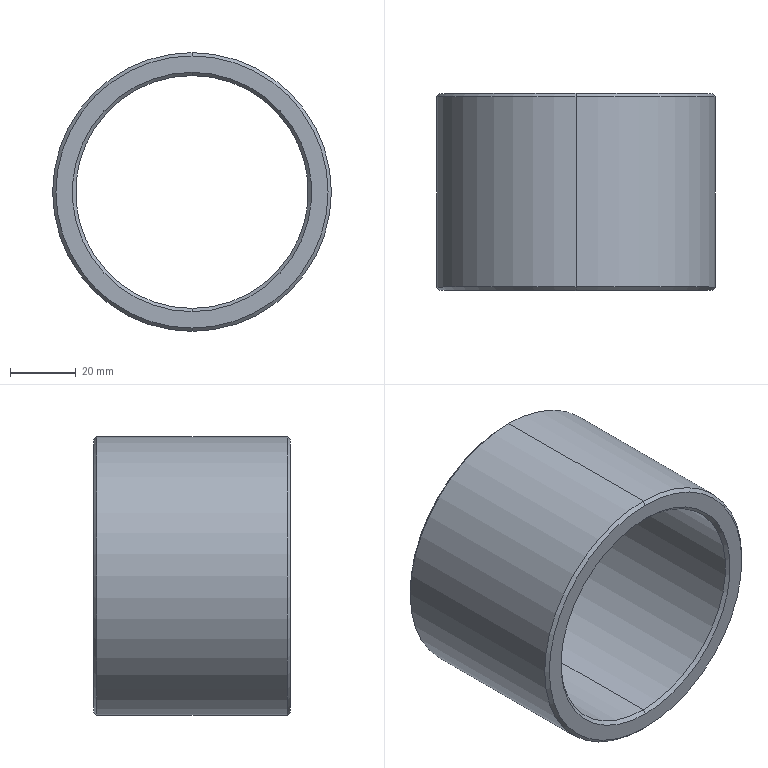Part | SolidWorks | features Chamfer 1, Extrusion 1 | 1 solid | 14 faces | box 85 x 60 x 85 mm | volume 102428 mm3 | cone 8 | cylinder 4 | plane 2 | commonest cylinder face diameters 71 x2 85 x2
STEP:
#1=CARTESIAN_POINT('',(0.,60.,41.5));
#2=VERTEX_POINT('',#1);
#3=CARTESIAN_POINT('',(0.,60.,-41.5));
#4=VERTEX_POINT('',#3);
#5=CARTESIAN_POINT('',(0.,60.,0.));
#6=DIRECTION('',(0.,1.,0.));
#7=DIRECTION('',(0.,0.,1.));
#8=AXIS2_PLACEMENT_3D('',#5,#6,#7);
#9=CIRCLE('',#8,41.5);
#10=EDGE_CURVE('',#2,#4,#9,.T.);
#11=ORIENTED_EDGE('',*,*,#10,.F.);
#12=CARTESIAN_POINT('',(0.,59.,42.5));
#13=VERTEX_POINT('',#12);
#14=CARTESIAN_POINT('',(0.,60.,41.5));
#15=DIRECTION('',(0.,-0.7071,0.7071));
#16=VECTOR('',#15,1000.);
#17=LINE('',#14,#16);
#18=EDGE_CURVE('',#2,#13,#17,.T.);
#19=ORIENTED_EDGE('',*,*,#18,.T.);
#20=CARTESIAN_POINT('',(0.,59.,-42.5));
#21=VERTEX_POINT('',#20);
#22=CARTESIAN_POINT('',(0.,59.,0.));
#23=DIRECTION('',(0.,-1.,0.));
#24=DIRECTION('',(0.,0.,1.));
#25=AXIS2_PLACEMENT_3D('',#22,#23,#24);
#26=CIRCLE('',#25,42.5);
#27=EDGE_CURVE('',#21,#13,#26,.T.);
#28=ORIENTED_EDGE('',*,*,#27,.F.);
#29=CARTESIAN_POINT('',(0.,60.,-41.5));
#30=DIRECTION('',(0.,-0.7071,-0.7071));
#31=VECTOR('',#30,1000.);
#32=LINE('',#29,#31);
#33=EDGE_CURVE('',#4,#21,#32,.T.);
#34=ORIENTED_EDGE('',*,*,#33,.F.);
#35=EDGE_LOOP('',(#11,#19,#28,#34));
#36=FACE_OUTER_BOUND('',#35,.T.);
#37=CARTESIAN_POINT('',(0.,60.,0.));
#38=DIRECTION('',(0.,-1.,0.));
#39=DIRECTION('',(0.,0.,-1.));
#40=AXIS2_PLACEMENT_3D('',#37,#38,#39);
#41=CONICAL_SURFACE('',#40,41.5,0.7854);
#42=ADVANCED_FACE('',(#36),#41,.T.);
#43=CARTESIAN_POINT('',(0.,0.,-41.5));
#44=VERTEX_POINT('',#43);
#45=CARTESIAN_POINT('',(0.,0.,41.5));
#46=VERTEX_POINT('',#45);
#47=CARTESIAN_POINT('',(0.,0.,0.));
#48=DIRECTION('',(0.,-1.,0.));
#49=DIRECTION('',(0.,0.,1.));
#50=AXIS2_PLACEMENT_3D('',#47,#48,#49);
#51=CIRCLE('',#50,41.5);
#52=EDGE_CURVE('',#44,#46,#51,.T.);
#53=ORIENTED_EDGE('',*,*,#52,.F.);
#54=CARTESIAN_POINT('',(0.,1.,-42.5));
#55=VERTEX_POINT('',#54);
#56=CARTESIAN_POINT('',(0.,1.,-42.5));
#57=DIRECTION('',(0.,0.7071,-0.7071));
#58=VECTOR('',#57,1000.);
#59=LINE('',#56,#58);
#60=EDGE_CURVE('',#44,#55,#59,.T.);
#61=ORIENTED_EDGE('',*,*,#60,.T.);
#62=CARTESIAN_POINT('',(0.,1.,42.5));
#63=VERTEX_POINT('',#62);
#64=CARTESIAN_POINT('',(0.,1.,0.));
#65=DIRECTION('',(0.,1.,0.));
#66=DIRECTION('',(0.,0.,1.));
#67=AXIS2_PLACEMENT_3D('',#64,#65,#66);
#68=CIRCLE('',#67,42.5);
#69=EDGE_CURVE('',#63,#55,#68,.T.);
#70=ORIENTED_EDGE('',*,*,#69,.F.);
#71=CARTESIAN_POINT('',(0.,1.,42.5));
#72=DIRECTION('',(0.,0.7071,0.7071));
#73=VECTOR('',#72,1000.);
#74=LINE('',#71,#73);
#75=EDGE_CURVE('',#46,#63,#74,.T.);
#76=ORIENTED_EDGE('',*,*,#75,.F.);
#77=EDGE_LOOP('',(#53,#61,#70,#76));
#78=FACE_OUTER_BOUND('',#77,.T.);
#79=CARTESIAN_POINT('',(0.,1.,0.));
#80=DIRECTION('',(0.,1.,0.));
#81=DIRECTION('',(0.,0.,1.));
#82=AXIS2_PLACEMENT_3D('',#79,#80,#81);
#83=CONICAL_SURFACE('',#82,42.5,0.7854);
#84=ADVANCED_FACE('',(#78),#83,.T.);
#85=CARTESIAN_POINT('',(0.,59.,-35.5));
#86=VERTEX_POINT('',#85);
#87=CARTESIAN_POINT('',(0.,59.,35.5));
#88=VERTEX_POINT('',#87);
#89=CARTESIAN_POINT('',(0.,59.,0.));
#90=DIRECTION('',(0.,1.,0.));
#91=DIRECTION('',(0.,0.,1.));
#92=AXIS2_PLACEMENT_3D('',#89,#90,#91);
#93=CIRCLE('',#92,35.5);
#94=EDGE_CURVE('',#86,#88,#93,.T.);
#95=ORIENTED_EDGE('',*,*,#94,.F.);
#96=CARTESIAN_POINT('',(0.,60.,-36.5));
#97=VERTEX_POINT('',#96);
#98=CARTESIAN_POINT('',(0.,59.,-35.5));
#99=DIRECTION('',(0.,0.7071,-0.7071));
#100=VECTOR('',#99,1000.);
#101=LINE('',#98,#100);
#102=EDGE_CURVE('',#86,#97,#101,.T.);
#103=ORIENTED_EDGE('',*,*,#102,.T.);
#104=CARTESIAN_POINT('',(0.,60.,36.5));
#105=VERTEX_POINT('',#104);
#106=CARTESIAN_POINT('',(0.,60.,0.));
#107=DIRECTION('',(0.,-1.,0.));
#108=DIRECTION('',(0.,0.,1.));
#109=AXIS2_PLACEMENT_3D('',#106,#107,#108);
#110=CIRCLE('',#109,36.5);
#111=EDGE_CURVE('',#105,#97,#110,.T.);
#112=ORIENTED_EDGE('',*,*,#111,.F.);
#113=CARTESIAN_POINT('',(0.,59.,35.5));
#114=DIRECTION('',(0.,0.7071,0.7071));
#115=VECTOR('',#114,1000.);
#116=LINE('',#113,#115);
#117=EDGE_CURVE('',#88,#105,#116,.T.);
#118=ORIENTED_EDGE('',*,*,#117,.F.);
#119=EDGE_LOOP('',(#95,#103,#112,#118));
#120=FACE_OUTER_BOUND('',#119,.T.);
#121=CARTESIAN_POINT('',(0.,59.,0.));
#122=DIRECTION('',(0.,1.,0.));
#123=DIRECTION('',(0.,0.,1.));
#124=AXIS2_PLACEMENT_3D('',#121,#122,#123);
#125=CONICAL_SURFACE('',#124,35.5,0.7854);
#126=ADVANCED_FACE('',(#120),#125,.F.);
#127=CARTESIAN_POINT('',(0.,1.,35.5));
#128=VERTEX_POINT('',#127);
#129=CARTESIAN_POINT('',(0.,1.,-35.5));
#130=VERTEX_POINT('',#129);
#131=CARTESIAN_POINT('',(0.,1.,0.));
#132=DIRECTION('',(0.,-1.,0.));
#133=DIRECTION('',(0.,0.,1.));
#134=AXIS2_PLACEMENT_3D('',#131,#132,#133);
#135=CIRCLE('',#134,35.5);
#136=EDGE_CURVE('',#128,#130,#135,.T.);
#137=ORIENTED_EDGE('',*,*,#136,.F.);
#138=CARTESIAN_POINT('',(0.,0.,36.5));
#139=VERTEX_POINT('',#138);
#140=CARTESIAN_POINT('',(0.,0.,36.5));
#141=DIRECTION('',(0.,-0.7071,0.7071));
#142=VECTOR('',#141,1000.);
#143=LINE('',#140,#142);
#144=EDGE_CURVE('',#128,#139,#143,.T.);
#145=ORIENTED_EDGE('',*,*,#144,.T.);
#146=CARTESIAN_POINT('',(0.,0.,-36.5));
#147=VERTEX_POINT('',#146);
#148=CARTESIAN_POINT('',(0.,0.,0.));
#149=DIRECTION('',(0.,1.,0.));
#150=DIRECTION('',(0.,0.,1.));
#151=AXIS2_PLACEMENT_3D('',#148,#149,#150);
#152=CIRCLE('',#151,36.5);
#153=EDGE_CURVE('',#147,#139,#152,.T.);
#154=ORIENTED_EDGE('',*,*,#153,.F.);
#155=CARTESIAN_POINT('',(0.,0.,-36.5));
#156=DIRECTION('',(0.,-0.7071,-0.7071));
#157=VECTOR('',#156,1000.);
#158=LINE('',#155,#157);
#159=EDGE_CURVE('',#130,#147,#158,.T.);
#160=ORIENTED_EDGE('',*,*,#159,.F.);
#161=EDGE_LOOP('',(#137,#145,#154,#160));
#162=FACE_OUTER_BOUND('',#161,.T.);
#163=CARTESIAN_POINT('',(0.,0.,0.));
#164=DIRECTION('',(0.,-1.,0.));
#165=DIRECTION('',(0.,0.,-1.));
#166=AXIS2_PLACEMENT_3D('',#163,#164,#165);
#167=CONICAL_SURFACE('',#166,36.5,0.7854);
#168=ADVANCED_FACE('',(#162),#167,.F.);
#169=ORIENTED_EDGE('',*,*,#94,.T.);
#170=CARTESIAN_POINT('',(0.,60.,35.5));
#171=DIRECTION('',(0.,-1.,0.));
#172=VECTOR('',#171,1000.);
#173=LINE('',#170,#172);
#174=EDGE_CURVE('',#88,#128,#173,.T.);
#175=ORIENTED_EDGE('',*,*,#174,.T.);
#176=ORIENTED_EDGE('',*,*,#136,.T.);
#177=CARTESIAN_POINT('',(0.,60.,-35.5));
#178=DIRECTION('',(0.,-1.,0.));
#179=VECTOR('',#178,1000.);
#180=LINE('',#177,#179);
#181=EDGE_CURVE('',#86,#130,#180,.T.);
#182=ORIENTED_EDGE('',*,*,#181,.F.);
#183=EDGE_LOOP('',(#169,#175,#176,#182));
#184=FACE_OUTER_BOUND('',#183,.T.);
#185=CARTESIAN_POINT('',(0.,60.,0.));
#186=DIRECTION('',(0.,-1.,0.));
#187=DIRECTION('',(0.,0.,-1.));
#188=AXIS2_PLACEMENT_3D('',#185,#186,#187);
#189=CYLINDRICAL_SURFACE('',#188,35.5);
#190=ADVANCED_FACE('',(#184),#189,.F.);
#191=ORIENTED_EDGE('',*,*,#27,.T.);
#192=CARTESIAN_POINT('',(0.,60.,42.5));
#193=DIRECTION('',(0.,-1.,0.));
#194=VECTOR('',#193,1000.);
#195=LINE('',#192,#194);
#196=EDGE_CURVE('',#13,#63,#195,.T.);
#197=ORIENTED_EDGE('',*,*,#196,.T.);
#198=ORIENTED_EDGE('',*,*,#69,.T.);
#199=CARTESIAN_POINT('',(0.,60.,-42.5));
#200=DIRECTION('',(0.,-1.,0.));
#201=VECTOR('',#200,1000.);
#202=LINE('',#199,#201);
#203=EDGE_CURVE('',#21,#55,#202,.T.);
#204=ORIENTED_EDGE('',*,*,#203,.F.);
#205=EDGE_LOOP('',(#191,#197,#198,#204));
#206=FACE_OUTER_BOUND('',#205,.T.);
#207=CARTESIAN_POINT('',(0.,60.,0.));
#208=DIRECTION('',(0.,-1.,0.));
#209=DIRECTION('',(0.,0.,-1.));
#210=AXIS2_PLACEMENT_3D('',#207,#208,#209);
#211=CYLINDRICAL_SURFACE('',#210,42.5);
#212=ADVANCED_FACE('',(#206),#211,.T.);
#213=ORIENTED_EDGE('',*,*,#111,.T.);
#214=CARTESIAN_POINT('',(0.,60.,0.));
#215=DIRECTION('',(0.,-1.,0.));
#216=DIRECTION('',(0.,0.,1.));
#217=AXIS2_PLACEMENT_3D('',#214,#215,#216);
#218=CIRCLE('',#217,36.5);
#219=EDGE_CURVE('',#97,#105,#218,.T.);
#220=ORIENTED_EDGE('',*,*,#219,.T.);
#221=EDGE_LOOP('',(#213,#220));
#222=FACE_BOUND('',#221,.T.);
#223=CARTESIAN_POINT('',(0.,60.,0.));
#224=DIRECTION('',(0.,1.,0.));
#225=DIRECTION('',(0.,0.,1.));
#226=AXIS2_PLACEMENT_3D('',#223,#224,#225);
#227=CIRCLE('',#226,41.5);
#228=EDGE_CURVE('',#4,#2,#227,.T.);
#229=ORIENTED_EDGE('',*,*,#228,.T.);
#230=ORIENTED_EDGE('',*,*,#10,.T.);
#231=EDGE_LOOP('',(#229,#230));
#232=FACE_OUTER_BOUND('',#231,.T.);
#233=CARTESIAN_POINT('',(0.,60.,0.));
#234=DIRECTION('',(0.,1.,0.));
#235=DIRECTION('',(0.,0.,1.));
#236=AXIS2_PLACEMENT_3D('',#233,#234,#235);
#237=PLANE('',#236);
#238=ADVANCED_FACE('',(#222,#232),#237,.T.);
#239=ORIENTED_EDGE('',*,*,#153,.T.);
#240=CARTESIAN_POINT('',(0.,0.,0.));
#241=DIRECTION('',(0.,1.,0.));
#242=DIRECTION('',(0.,0.,1.));
#243=AXIS2_PLACEMENT_3D('',#240,#241,#242);
#244=CIRCLE('',#243,36.5);
#245=EDGE_CURVE('',#139,#147,#244,.T.);
#246=ORIENTED_EDGE('',*,*,#245,.T.);
#247=EDGE_LOOP('',(#239,#246));
#248=FACE_BOUND('',#247,.T.);
#249=CARTESIAN_POINT('',(0.,0.,0.));
#250=DIRECTION('',(0.,-1.,0.));
#251=DIRECTION('',(0.,0.,1.));
#252=AXIS2_PLACEMENT_3D('',#249,#250,#251);
#253=CIRCLE('',#252,41.5);
#254=EDGE_CURVE('',#46,#44,#253,.T.);
#255=ORIENTED_EDGE('',*,*,#254,.T.);
#256=ORIENTED_EDGE('',*,*,#52,.T.);
#257=EDGE_LOOP('',(#255,#256));
#258=FACE_OUTER_BOUND('',#257,.T.);
#259=CARTESIAN_POINT('',(0.,0.,0.));
#260=DIRECTION('',(0.,1.,0.));
#261=DIRECTION('',(0.,0.,1.));
#262=AXIS2_PLACEMENT_3D('',#259,#260,#261);
#263=PLANE('',#262);
#264=ADVANCED_FACE('',(#248,#258),#263,.F.);
#265=ORIENTED_EDGE('',*,*,#196,.F.);
#266=CARTESIAN_POINT('',(0.,59.,0.));
#267=DIRECTION('',(0.,-1.,0.));
#268=DIRECTION('',(0.,0.,1.));
#269=AXIS2_PLACEMENT_3D('',#266,#267,#268);
#270=CIRCLE('',#269,42.5);
#271=EDGE_CURVE('',#13,#21,#270,.T.);
#272=ORIENTED_EDGE('',*,*,#271,.T.);
#273=ORIENTED_EDGE('',*,*,#203,.T.);
#274=CARTESIAN_POINT('',(0.,1.,0.));
#275=DIRECTION('',(0.,1.,0.));
#276=DIRECTION('',(0.,0.,1.));
#277=AXIS2_PLACEMENT_3D('',#274,#275,#276);
#278=CIRCLE('',#277,42.5);
#279=EDGE_CURVE('',#55,#63,#278,.T.);
#280=ORIENTED_EDGE('',*,*,#279,.T.);
#281=EDGE_LOOP('',(#265,#272,#273,#280));
#282=FACE_OUTER_BOUND('',#281,.T.);
#283=CARTESIAN_POINT('',(0.,60.,0.));
#284=DIRECTION('',(0.,-1.,0.));
#285=DIRECTION('',(0.,0.,-1.));
#286=AXIS2_PLACEMENT_3D('',#283,#284,#285);
#287=CYLINDRICAL_SURFACE('',#286,42.5);
#288=ADVANCED_FACE('',(#282),#287,.T.);
#289=ORIENTED_EDGE('',*,*,#174,.F.);
#290=CARTESIAN_POINT('',(0.,59.,0.));
#291=DIRECTION('',(0.,1.,0.));
#292=DIRECTION('',(0.,0.,1.));
#293=AXIS2_PLACEMENT_3D('',#290,#291,#292);
#294=CIRCLE('',#293,35.5);
#295=EDGE_CURVE('',#88,#86,#294,.T.);
#296=ORIENTED_EDGE('',*,*,#295,.T.);
#297=ORIENTED_EDGE('',*,*,#181,.T.);
#298=CARTESIAN_POINT('',(0.,1.,0.));
#299=DIRECTION('',(0.,-1.,0.));
#300=DIRECTION('',(0.,0.,1.));
#301=AXIS2_PLACEMENT_3D('',#298,#299,#300);
#302=CIRCLE('',#301,35.5);
#303=EDGE_CURVE('',#130,#128,#302,.T.);
#304=ORIENTED_EDGE('',*,*,#303,.T.);
#305=EDGE_LOOP('',(#289,#296,#297,#304));
#306=FACE_OUTER_BOUND('',#305,.T.);
#307=CARTESIAN_POINT('',(0.,60.,0.));
#308=DIRECTION('',(0.,-1.,0.));
#309=DIRECTION('',(0.,0.,-1.));
#310=AXIS2_PLACEMENT_3D('',#307,#308,#309);
#311=CYLINDRICAL_SURFACE('',#310,35.5);
#312=ADVANCED_FACE('',(#306),#311,.F.);
#313=ORIENTED_EDGE('',*,*,#144,.F.);
#314=ORIENTED_EDGE('',*,*,#303,.F.);
#315=ORIENTED_EDGE('',*,*,#159,.T.);
#316=ORIENTED_EDGE('',*,*,#245,.F.);
#317=EDGE_LOOP('',(#313,#314,#315,#316));
#318=FACE_OUTER_BOUND('',#317,.T.);
#319=CARTESIAN_POINT('',(0.,0.,0.));
#320=DIRECTION('',(0.,-1.,0.));
#321=DIRECTION('',(0.,0.,-1.));
#322=AXIS2_PLACEMENT_3D('',#319,#320,#321);
#323=CONICAL_SURFACE('',#322,36.5,0.7854);
#324=ADVANCED_FACE('',(#318),#323,.F.);
#325=ORIENTED_EDGE('',*,*,#102,.F.);
#326=ORIENTED_EDGE('',*,*,#295,.F.);
#327=ORIENTED_EDGE('',*,*,#117,.T.);
#328=ORIENTED_EDGE('',*,*,#219,.F.);
#329=EDGE_LOOP('',(#325,#326,#327,#328));
#330=FACE_OUTER_BOUND('',#329,.T.);
#331=CARTESIAN_POINT('',(0.,59.,0.));
#332=DIRECTION('',(0.,1.,0.));
#333=DIRECTION('',(0.,0.,1.));
#334=AXIS2_PLACEMENT_3D('',#331,#332,#333);
#335=CONICAL_SURFACE('',#334,35.5,0.7854);
#336=ADVANCED_FACE('',(#330),#335,.F.);
#337=ORIENTED_EDGE('',*,*,#60,.F.);
#338=ORIENTED_EDGE('',*,*,#254,.F.);
#339=ORIENTED_EDGE('',*,*,#75,.T.);
#340=ORIENTED_EDGE('',*,*,#279,.F.);
#341=EDGE_LOOP('',(#337,#338,#339,#340));
#342=FACE_OUTER_BOUND('',#341,.T.);
#343=CARTESIAN_POINT('',(0.,1.,0.));
#344=DIRECTION('',(0.,1.,0.));
#345=DIRECTION('',(0.,0.,1.));
#346=AXIS2_PLACEMENT_3D('',#343,#344,#345);
#347=CONICAL_SURFACE('',#346,42.5,0.7854);
#348=ADVANCED_FACE('',(#342),#347,.T.);
#349=ORIENTED_EDGE('',*,*,#18,.F.);
#350=ORIENTED_EDGE('',*,*,#228,.F.);
#351=ORIENTED_EDGE('',*,*,#33,.T.);
#352=ORIENTED_EDGE('',*,*,#271,.F.);
#353=EDGE_LOOP('',(#349,#350,#351,#352));
#354=FACE_OUTER_BOUND('',#353,.T.);
#355=CARTESIAN_POINT('',(0.,60.,0.));
#356=DIRECTION('',(0.,-1.,0.));
#357=DIRECTION('',(0.,0.,-1.));
#358=AXIS2_PLACEMENT_3D('',#355,#356,#357);
#359=CONICAL_SURFACE('',#358,41.5,0.7854);
#360=ADVANCED_FACE('',(#354),#359,.T.);
#361=CLOSED_SHELL('',(#42,#84,#126,#168,#190,#212,#238,#264,#288,#312,#324,#336,#348,#360));
#362=MANIFOLD_SOLID_BREP('',#361);
#363=CARTESIAN_POINT('',(0.,0.,0.));
#364=DIRECTION('',(0.,0.,1.));
#365=DIRECTION('',(1.,0.,0.));
#366=AXIS2_PLACEMENT_3D('',#363,#364,#365);
#367=(LENGTH_UNIT()NAMED_UNIT(*)SI_UNIT(.MILLI.,.METRE.));
#368=UNCERTAINTY_MEASURE_WITH_UNIT(LENGTH_MEASURE(0.00001),#367,'','');
#369=(NAMED_UNIT(*)PLANE_ANGLE_UNIT()SI_UNIT($,.RADIAN.));
#370=(NAMED_UNIT(*)SI_UNIT($,.STERADIAN.)SOLID_ANGLE_UNIT());
#371=(GEOMETRIC_REPRESENTATION_CONTEXT(3)GLOBAL_UNCERTAINTY_ASSIGNED_CONTEXT((#368))GLOBAL_UNIT_ASSIGNED_CONTEXT((#367,#369,#370))REPRESENTATION_CONTEXT('',''));
#372=ADVANCED_BREP_SHAPE_REPRESENTATION('',(#362,#366),#371);